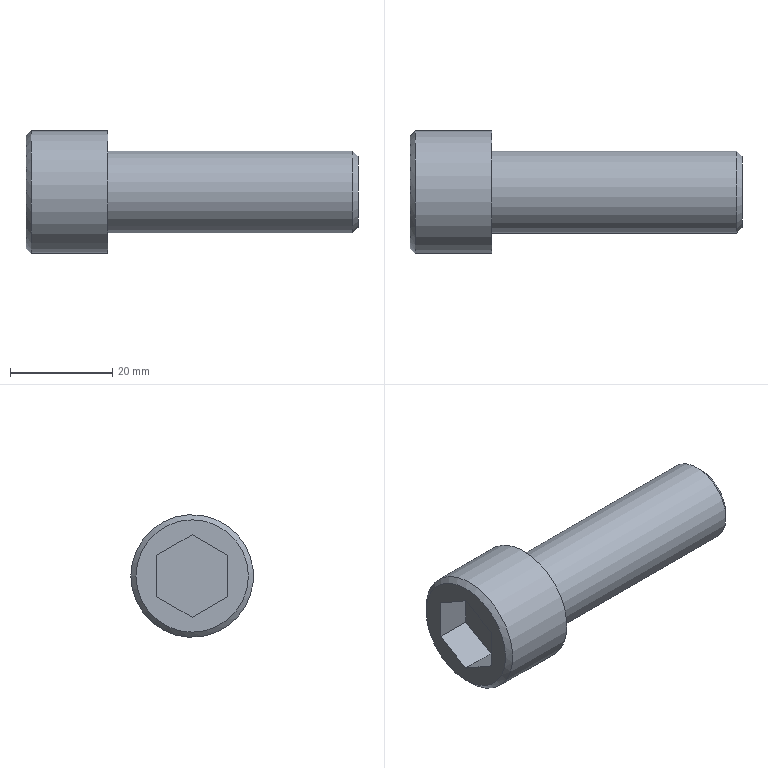Part | STEP file | solid 63 | 1 solid | 14 faces | box 65 x 24 x 24 mm | volume 15841 mm3 | plane 10 | cylinder 2 | cone 2 | commonest cylinder face diameters 16 x1 24 x1